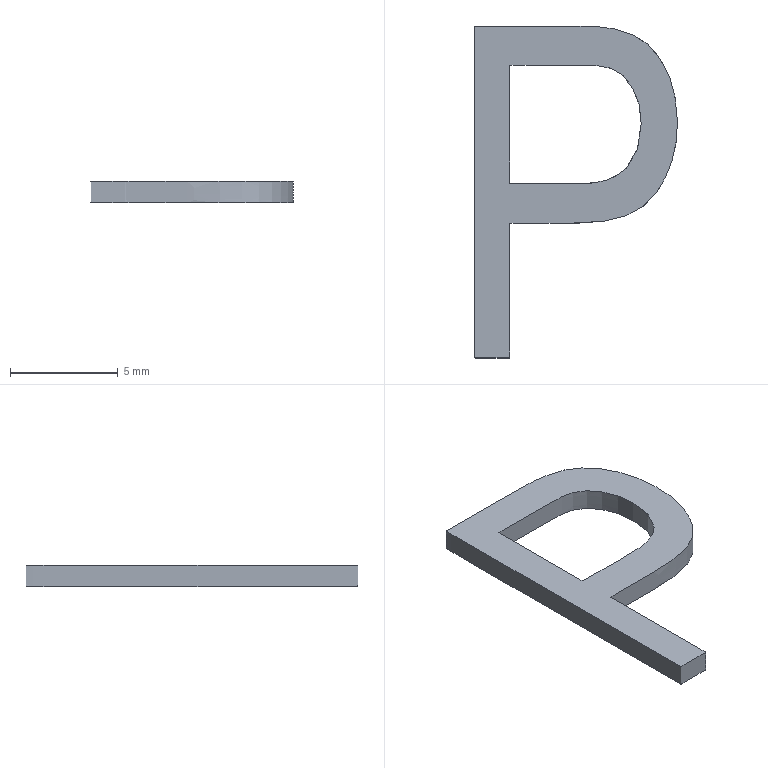Part | STEP file | lll_id970_x_t | 1 solid | 4 faces | box 9.426 x 15.432 x 1 mm | volume 57.711 mm3 | other 2 | plane 2